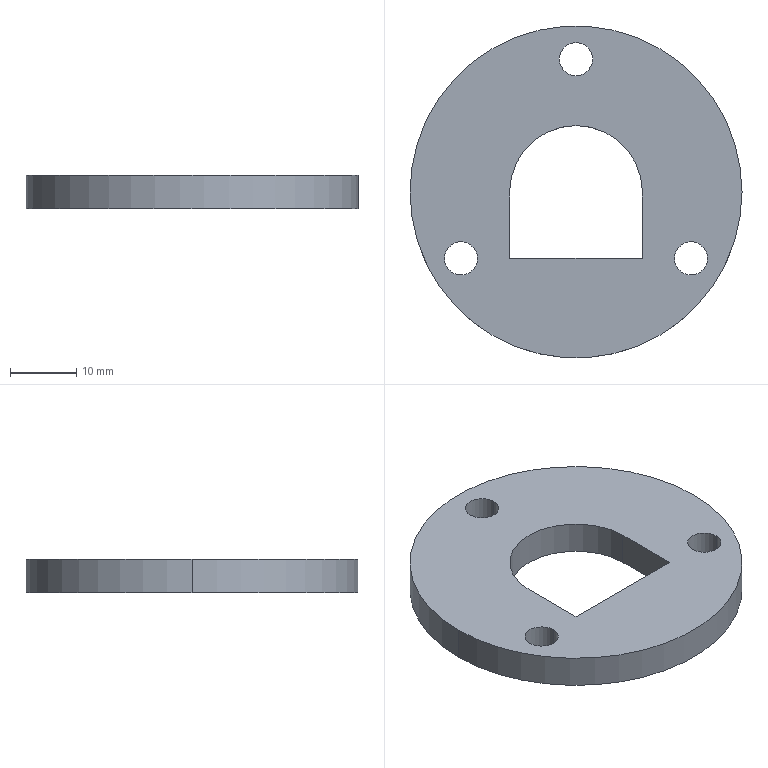Part | SolidWorks | features BaseBody 1 | 1 solid | 14 faces | box 50 x 50 x 5 mm | volume 7738 mm3 | cylinder 9 | plane 5 | commonest cylinder face diameters 5 x6 50 x2 20 x1
STEP:
#1=CARTESIAN_POINT('',(19.821,-10.,0.));
#2=VERTEX_POINT('',#1);
#3=CARTESIAN_POINT('',(14.821,-10.,0.));
#4=VERTEX_POINT('',#3);
#5=CARTESIAN_POINT('',(17.321,-10.,0.));
#6=DIRECTION('',(0.,0.,1.));
#7=DIRECTION('',(-1.,0.,0.));
#8=AXIS2_PLACEMENT_3D('',#5,#6,#7);
#9=CIRCLE('',#8,2.5);
#10=EDGE_CURVE('',#2,#4,#9,.T.);
#11=ORIENTED_EDGE('',*,*,#10,.F.);
#12=CARTESIAN_POINT('',(19.821,-10.,5.));
#13=VERTEX_POINT('',#12);
#14=CARTESIAN_POINT('',(19.821,-10.,5.));
#15=DIRECTION('',(0.,0.,1.));
#16=VECTOR('',#15,1000.);
#17=LINE('',#14,#16);
#18=EDGE_CURVE('',#2,#13,#17,.T.);
#19=ORIENTED_EDGE('',*,*,#18,.T.);
#20=CARTESIAN_POINT('',(14.821,-10.,5.));
#21=VERTEX_POINT('',#20);
#22=CARTESIAN_POINT('',(17.321,-10.,5.));
#23=DIRECTION('',(0.,0.,-1.));
#24=DIRECTION('',(-1.,0.,0.));
#25=AXIS2_PLACEMENT_3D('',#22,#23,#24);
#26=CIRCLE('',#25,2.5);
#27=EDGE_CURVE('',#21,#13,#26,.T.);
#28=ORIENTED_EDGE('',*,*,#27,.F.);
#29=CARTESIAN_POINT('',(14.821,-10.,5.));
#30=DIRECTION('',(0.,0.,1.));
#31=VECTOR('',#30,1000.);
#32=LINE('',#29,#31);
#33=EDGE_CURVE('',#4,#21,#32,.T.);
#34=ORIENTED_EDGE('',*,*,#33,.F.);
#35=EDGE_LOOP('',(#11,#19,#28,#34));
#36=FACE_OUTER_BOUND('',#35,.T.);
#37=CARTESIAN_POINT('',(17.321,-10.,5.));
#38=DIRECTION('',(0.,0.,1.));
#39=DIRECTION('',(-1.,0.,0.));
#40=AXIS2_PLACEMENT_3D('',#37,#38,#39);
#41=CYLINDRICAL_SURFACE('',#40,2.5);
#42=ADVANCED_FACE('',(#36),#41,.F.);
#43=CARTESIAN_POINT('',(-14.821,-10.,0.));
#44=VERTEX_POINT('',#43);
#45=CARTESIAN_POINT('',(-19.821,-10.,0.));
#46=VERTEX_POINT('',#45);
#47=CARTESIAN_POINT('',(-17.321,-10.,0.));
#48=DIRECTION('',(0.,0.,1.));
#49=DIRECTION('',(-1.,0.,0.));
#50=AXIS2_PLACEMENT_3D('',#47,#48,#49);
#51=CIRCLE('',#50,2.5);
#52=EDGE_CURVE('',#44,#46,#51,.T.);
#53=ORIENTED_EDGE('',*,*,#52,.F.);
#54=CARTESIAN_POINT('',(-14.821,-10.,5.));
#55=VERTEX_POINT('',#54);
#56=CARTESIAN_POINT('',(-14.821,-10.,5.));
#57=DIRECTION('',(0.,0.,1.));
#58=VECTOR('',#57,1000.);
#59=LINE('',#56,#58);
#60=EDGE_CURVE('',#44,#55,#59,.T.);
#61=ORIENTED_EDGE('',*,*,#60,.T.);
#62=CARTESIAN_POINT('',(-19.821,-10.,5.));
#63=VERTEX_POINT('',#62);
#64=CARTESIAN_POINT('',(-17.321,-10.,5.));
#65=DIRECTION('',(0.,0.,-1.));
#66=DIRECTION('',(-1.,0.,0.));
#67=AXIS2_PLACEMENT_3D('',#64,#65,#66);
#68=CIRCLE('',#67,2.5);
#69=EDGE_CURVE('',#63,#55,#68,.T.);
#70=ORIENTED_EDGE('',*,*,#69,.F.);
#71=CARTESIAN_POINT('',(-19.821,-10.,5.));
#72=DIRECTION('',(0.,0.,1.));
#73=VECTOR('',#72,1000.);
#74=LINE('',#71,#73);
#75=EDGE_CURVE('',#46,#63,#74,.T.);
#76=ORIENTED_EDGE('',*,*,#75,.F.);
#77=EDGE_LOOP('',(#53,#61,#70,#76));
#78=FACE_OUTER_BOUND('',#77,.T.);
#79=CARTESIAN_POINT('',(-17.321,-10.,5.));
#80=DIRECTION('',(0.,0.,1.));
#81=DIRECTION('',(-1.,0.,0.));
#82=AXIS2_PLACEMENT_3D('',#79,#80,#81);
#83=CYLINDRICAL_SURFACE('',#82,2.5);
#84=ADVANCED_FACE('',(#78),#83,.F.);
#85=CARTESIAN_POINT('',(2.5,20.,0.));
#86=VERTEX_POINT('',#85);
#87=CARTESIAN_POINT('',(-2.5,20.,0.));
#88=VERTEX_POINT('',#87);
#89=CARTESIAN_POINT('',(0.,20.,0.));
#90=DIRECTION('',(0.,0.,1.));
#91=DIRECTION('',(-1.,0.,0.));
#92=AXIS2_PLACEMENT_3D('',#89,#90,#91);
#93=CIRCLE('',#92,2.5);
#94=EDGE_CURVE('',#86,#88,#93,.T.);
#95=ORIENTED_EDGE('',*,*,#94,.F.);
#96=CARTESIAN_POINT('',(2.5,20.,5.));
#97=VERTEX_POINT('',#96);
#98=CARTESIAN_POINT('',(2.5,20.,5.));
#99=DIRECTION('',(0.,0.,1.));
#100=VECTOR('',#99,1000.);
#101=LINE('',#98,#100);
#102=EDGE_CURVE('',#86,#97,#101,.T.);
#103=ORIENTED_EDGE('',*,*,#102,.T.);
#104=CARTESIAN_POINT('',(-2.5,20.,5.));
#105=VERTEX_POINT('',#104);
#106=CARTESIAN_POINT('',(0.,20.,5.));
#107=DIRECTION('',(0.,0.,-1.));
#108=DIRECTION('',(-1.,0.,0.));
#109=AXIS2_PLACEMENT_3D('',#106,#107,#108);
#110=CIRCLE('',#109,2.5);
#111=EDGE_CURVE('',#105,#97,#110,.T.);
#112=ORIENTED_EDGE('',*,*,#111,.F.);
#113=CARTESIAN_POINT('',(-2.5,20.,5.));
#114=DIRECTION('',(0.,0.,1.));
#115=VECTOR('',#114,1000.);
#116=LINE('',#113,#115);
#117=EDGE_CURVE('',#88,#105,#116,.T.);
#118=ORIENTED_EDGE('',*,*,#117,.F.);
#119=EDGE_LOOP('',(#95,#103,#112,#118));
#120=FACE_OUTER_BOUND('',#119,.T.);
#121=CARTESIAN_POINT('',(0.,20.,5.));
#122=DIRECTION('',(0.,0.,1.));
#123=DIRECTION('',(-1.,0.,0.));
#124=AXIS2_PLACEMENT_3D('',#121,#122,#123);
#125=CYLINDRICAL_SURFACE('',#124,2.5);
#126=ADVANCED_FACE('',(#120),#125,.F.);
#127=CARTESIAN_POINT('',(25.,0.,5.));
#128=VERTEX_POINT('',#127);
#129=CARTESIAN_POINT('',(-25.,0.,5.));
#130=VERTEX_POINT('',#129);
#131=CARTESIAN_POINT('',(0.,0.,5.));
#132=DIRECTION('',(0.,0.,1.));
#133=DIRECTION('',(-1.,0.,0.));
#134=AXIS2_PLACEMENT_3D('',#131,#132,#133);
#135=CIRCLE('',#134,25.);
#136=EDGE_CURVE('',#128,#130,#135,.T.);
#137=ORIENTED_EDGE('',*,*,#136,.F.);
#138=CARTESIAN_POINT('',(25.,0.,0.));
#139=VERTEX_POINT('',#138);
#140=CARTESIAN_POINT('',(25.,0.,0.));
#141=DIRECTION('',(0.,0.,-1.));
#142=VECTOR('',#141,1000.);
#143=LINE('',#140,#142);
#144=EDGE_CURVE('',#128,#139,#143,.T.);
#145=ORIENTED_EDGE('',*,*,#144,.T.);
#146=CARTESIAN_POINT('',(-25.,0.,0.));
#147=VERTEX_POINT('',#146);
#148=CARTESIAN_POINT('',(0.,0.,0.));
#149=DIRECTION('',(0.,0.,-1.));
#150=DIRECTION('',(-1.,0.,0.));
#151=AXIS2_PLACEMENT_3D('',#148,#149,#150);
#152=CIRCLE('',#151,25.);
#153=EDGE_CURVE('',#147,#139,#152,.T.);
#154=ORIENTED_EDGE('',*,*,#153,.F.);
#155=CARTESIAN_POINT('',(-25.,0.,0.));
#156=DIRECTION('',(0.,0.,-1.));
#157=VECTOR('',#156,1000.);
#158=LINE('',#155,#157);
#159=EDGE_CURVE('',#130,#147,#158,.T.);
#160=ORIENTED_EDGE('',*,*,#159,.F.);
#161=EDGE_LOOP('',(#137,#145,#154,#160));
#162=FACE_OUTER_BOUND('',#161,.T.);
#163=CARTESIAN_POINT('',(0.,0.,0.));
#164=DIRECTION('',(0.,0.,-1.));
#165=DIRECTION('',(-1.,0.,0.));
#166=AXIS2_PLACEMENT_3D('',#163,#164,#165);
#167=CYLINDRICAL_SURFACE('',#166,25.);
#168=ADVANCED_FACE('',(#162),#167,.T.);
#169=CARTESIAN_POINT('',(10.,0.,0.));
#170=VERTEX_POINT('',#169);
#171=CARTESIAN_POINT('',(-10.,0.,0.));
#172=VERTEX_POINT('',#171);
#173=CARTESIAN_POINT('',(0.,0.,0.));
#174=DIRECTION('',(0.,0.,1.));
#175=DIRECTION('',(1.,0.,0.));
#176=AXIS2_PLACEMENT_3D('',#173,#174,#175);
#177=CIRCLE('',#176,10.);
#178=EDGE_CURVE('',#170,#172,#177,.T.);
#179=ORIENTED_EDGE('',*,*,#178,.F.);
#180=CARTESIAN_POINT('',(10.,0.,5.));
#181=VERTEX_POINT('',#180);
#182=CARTESIAN_POINT('',(10.,0.,5.));
#183=DIRECTION('',(0.,0.,-1.));
#184=VECTOR('',#183,1000.);
#185=LINE('',#182,#184);
#186=EDGE_CURVE('',#181,#170,#185,.T.);
#187=ORIENTED_EDGE('',*,*,#186,.F.);
#188=CARTESIAN_POINT('',(-10.,0.,5.));
#189=VERTEX_POINT('',#188);
#190=CARTESIAN_POINT('',(0.,0.,5.));
#191=DIRECTION('',(0.,0.,-1.));
#192=DIRECTION('',(1.,0.,0.));
#193=AXIS2_PLACEMENT_3D('',#190,#191,#192);
#194=CIRCLE('',#193,10.);
#195=EDGE_CURVE('',#189,#181,#194,.T.);
#196=ORIENTED_EDGE('',*,*,#195,.F.);
#197=CARTESIAN_POINT('',(-10.,0.,5.));
#198=DIRECTION('',(0.,0.,-1.));
#199=VECTOR('',#198,1000.);
#200=LINE('',#197,#199);
#201=EDGE_CURVE('',#189,#172,#200,.T.);
#202=ORIENTED_EDGE('',*,*,#201,.T.);
#203=EDGE_LOOP('',(#179,#187,#196,#202));
#204=FACE_OUTER_BOUND('',#203,.T.);
#205=CARTESIAN_POINT('',(0.,0.,5.));
#206=DIRECTION('',(0.,0.,1.));
#207=DIRECTION('',(1.,0.,0.));
#208=AXIS2_PLACEMENT_3D('',#205,#206,#207);
#209=CYLINDRICAL_SURFACE('',#208,10.);
#210=ADVANCED_FACE('',(#204),#209,.F.);
#211=CARTESIAN_POINT('',(-10.,-10.,0.));
#212=VERTEX_POINT('',#211);
#213=CARTESIAN_POINT('',(-10.,-5.,0.));
#214=DIRECTION('',(0.,-1.,0.));
#215=VECTOR('',#214,1000.);
#216=LINE('',#213,#215);
#217=EDGE_CURVE('',#172,#212,#216,.T.);
#218=ORIENTED_EDGE('',*,*,#217,.F.);
#219=ORIENTED_EDGE('',*,*,#201,.F.);
#220=CARTESIAN_POINT('',(-10.,-10.,5.));
#221=VERTEX_POINT('',#220);
#222=CARTESIAN_POINT('',(-10.,-5.,5.));
#223=DIRECTION('',(0.,1.,0.));
#224=VECTOR('',#223,1000.);
#225=LINE('',#222,#224);
#226=EDGE_CURVE('',#221,#189,#225,.T.);
#227=ORIENTED_EDGE('',*,*,#226,.F.);
#228=CARTESIAN_POINT('',(-10.,-10.,5.));
#229=DIRECTION('',(0.,0.,-1.));
#230=VECTOR('',#229,1000.);
#231=LINE('',#228,#230);
#232=EDGE_CURVE('',#221,#212,#231,.T.);
#233=ORIENTED_EDGE('',*,*,#232,.T.);
#234=EDGE_LOOP('',(#218,#219,#227,#233));
#235=FACE_OUTER_BOUND('',#234,.T.);
#236=CARTESIAN_POINT('',(-10.,-10.,5.));
#237=DIRECTION('',(-1.,0.,0.));
#238=DIRECTION('',(0.,0.,1.));
#239=AXIS2_PLACEMENT_3D('',#236,#237,#238);
#240=PLANE('',#239);
#241=ADVANCED_FACE('',(#235),#240,.F.);
#242=CARTESIAN_POINT('',(10.,-10.,0.));
#243=VERTEX_POINT('',#242);
#244=CARTESIAN_POINT('',(5.,-10.,0.));
#245=DIRECTION('',(1.,0.,0.));
#246=VECTOR('',#245,1000.);
#247=LINE('',#244,#246);
#248=EDGE_CURVE('',#212,#243,#247,.T.);
#249=ORIENTED_EDGE('',*,*,#248,.F.);
#250=ORIENTED_EDGE('',*,*,#232,.F.);
#251=CARTESIAN_POINT('',(10.,-10.,5.));
#252=VERTEX_POINT('',#251);
#253=CARTESIAN_POINT('',(5.,-10.,5.));
#254=DIRECTION('',(-1.,0.,0.));
#255=VECTOR('',#254,1000.);
#256=LINE('',#253,#255);
#257=EDGE_CURVE('',#252,#221,#256,.T.);
#258=ORIENTED_EDGE('',*,*,#257,.F.);
#259=CARTESIAN_POINT('',(10.,-10.,5.));
#260=DIRECTION('',(0.,0.,-1.));
#261=VECTOR('',#260,1000.);
#262=LINE('',#259,#261);
#263=EDGE_CURVE('',#252,#243,#262,.T.);
#264=ORIENTED_EDGE('',*,*,#263,.T.);
#265=EDGE_LOOP('',(#249,#250,#258,#264));
#266=FACE_OUTER_BOUND('',#265,.T.);
#267=CARTESIAN_POINT('',(10.,-10.,5.));
#268=DIRECTION('',(0.,-1.,0.));
#269=DIRECTION('',(0.,0.,-1.));
#270=AXIS2_PLACEMENT_3D('',#267,#268,#269);
#271=PLANE('',#270);
#272=ADVANCED_FACE('',(#266),#271,.F.);
#273=CARTESIAN_POINT('',(10.,0.,0.));
#274=DIRECTION('',(0.,1.,0.));
#275=VECTOR('',#274,1000.);
#276=LINE('',#273,#275);
#277=EDGE_CURVE('',#243,#170,#276,.T.);
#278=ORIENTED_EDGE('',*,*,#277,.F.);
#279=ORIENTED_EDGE('',*,*,#263,.F.);
#280=CARTESIAN_POINT('',(10.,0.,5.));
#281=DIRECTION('',(0.,-1.,0.));
#282=VECTOR('',#281,1000.);
#283=LINE('',#280,#282);
#284=EDGE_CURVE('',#181,#252,#283,.T.);
#285=ORIENTED_EDGE('',*,*,#284,.F.);
#286=ORIENTED_EDGE('',*,*,#186,.T.);
#287=EDGE_LOOP('',(#278,#279,#285,#286));
#288=FACE_OUTER_BOUND('',#287,.T.);
#289=CARTESIAN_POINT('',(10.,0.,5.));
#290=DIRECTION('',(1.,0.,0.));
#291=DIRECTION('',(0.,1.,0.));
#292=AXIS2_PLACEMENT_3D('',#289,#290,#291);
#293=PLANE('',#292);
#294=ADVANCED_FACE('',(#288),#293,.F.);
#295=CARTESIAN_POINT('',(17.321,-10.,0.));
#296=DIRECTION('',(0.,0.,1.));
#297=DIRECTION('',(-1.,0.,0.));
#298=AXIS2_PLACEMENT_3D('',#295,#296,#297);
#299=CIRCLE('',#298,2.5);
#300=EDGE_CURVE('',#4,#2,#299,.T.);
#301=ORIENTED_EDGE('',*,*,#300,.T.);
#302=ORIENTED_EDGE('',*,*,#10,.T.);
#303=EDGE_LOOP('',(#301,#302));
#304=FACE_BOUND('',#303,.T.);
#305=CARTESIAN_POINT('',(-17.321,-10.,0.));
#306=DIRECTION('',(0.,0.,1.));
#307=DIRECTION('',(-1.,0.,0.));
#308=AXIS2_PLACEMENT_3D('',#305,#306,#307);
#309=CIRCLE('',#308,2.5);
#310=EDGE_CURVE('',#46,#44,#309,.T.);
#311=ORIENTED_EDGE('',*,*,#310,.T.);
#312=ORIENTED_EDGE('',*,*,#52,.T.);
#313=EDGE_LOOP('',(#311,#312));
#314=FACE_BOUND('',#313,.T.);
#315=CARTESIAN_POINT('',(0.,20.,0.));
#316=DIRECTION('',(0.,0.,1.));
#317=DIRECTION('',(-1.,0.,0.));
#318=AXIS2_PLACEMENT_3D('',#315,#316,#317);
#319=CIRCLE('',#318,2.5);
#320=EDGE_CURVE('',#88,#86,#319,.T.);
#321=ORIENTED_EDGE('',*,*,#320,.T.);
#322=ORIENTED_EDGE('',*,*,#94,.T.);
#323=EDGE_LOOP('',(#321,#322));
#324=FACE_BOUND('',#323,.T.);
#325=ORIENTED_EDGE('',*,*,#248,.T.);
#326=ORIENTED_EDGE('',*,*,#277,.T.);
#327=ORIENTED_EDGE('',*,*,#178,.T.);
#328=ORIENTED_EDGE('',*,*,#217,.T.);
#329=EDGE_LOOP('',(#325,#326,#327,#328));
#330=FACE_BOUND('',#329,.T.);
#331=ORIENTED_EDGE('',*,*,#153,.T.);
#332=CARTESIAN_POINT('',(0.,0.,0.));
#333=DIRECTION('',(0.,0.,-1.));
#334=DIRECTION('',(-1.,0.,0.));
#335=AXIS2_PLACEMENT_3D('',#332,#333,#334);
#336=CIRCLE('',#335,25.);
#337=EDGE_CURVE('',#139,#147,#336,.T.);
#338=ORIENTED_EDGE('',*,*,#337,.T.);
#339=EDGE_LOOP('',(#331,#338));
#340=FACE_OUTER_BOUND('',#339,.T.);
#341=CARTESIAN_POINT('',(0.,0.,0.));
#342=DIRECTION('',(0.,0.,1.));
#343=DIRECTION('',(1.,0.,0.));
#344=AXIS2_PLACEMENT_3D('',#341,#342,#343);
#345=PLANE('',#344);
#346=ADVANCED_FACE('',(#304,#314,#324,#330,#340),#345,.F.);
#347=ORIENTED_EDGE('',*,*,#27,.T.);
#348=CARTESIAN_POINT('',(17.321,-10.,5.));
#349=DIRECTION('',(0.,0.,-1.));
#350=DIRECTION('',(-1.,0.,0.));
#351=AXIS2_PLACEMENT_3D('',#348,#349,#350);
#352=CIRCLE('',#351,2.5);
#353=EDGE_CURVE('',#13,#21,#352,.T.);
#354=ORIENTED_EDGE('',*,*,#353,.T.);
#355=EDGE_LOOP('',(#347,#354));
#356=FACE_BOUND('',#355,.T.);
#357=ORIENTED_EDGE('',*,*,#69,.T.);
#358=CARTESIAN_POINT('',(-17.321,-10.,5.));
#359=DIRECTION('',(0.,0.,-1.));
#360=DIRECTION('',(-1.,0.,0.));
#361=AXIS2_PLACEMENT_3D('',#358,#359,#360);
#362=CIRCLE('',#361,2.5);
#363=EDGE_CURVE('',#55,#63,#362,.T.);
#364=ORIENTED_EDGE('',*,*,#363,.T.);
#365=EDGE_LOOP('',(#357,#364));
#366=FACE_BOUND('',#365,.T.);
#367=ORIENTED_EDGE('',*,*,#111,.T.);
#368=CARTESIAN_POINT('',(0.,20.,5.));
#369=DIRECTION('',(0.,0.,-1.));
#370=DIRECTION('',(-1.,0.,0.));
#371=AXIS2_PLACEMENT_3D('',#368,#369,#370);
#372=CIRCLE('',#371,2.5);
#373=EDGE_CURVE('',#97,#105,#372,.T.);
#374=ORIENTED_EDGE('',*,*,#373,.T.);
#375=EDGE_LOOP('',(#367,#374));
#376=FACE_BOUND('',#375,.T.);
#377=ORIENTED_EDGE('',*,*,#257,.T.);
#378=ORIENTED_EDGE('',*,*,#226,.T.);
#379=ORIENTED_EDGE('',*,*,#195,.T.);
#380=ORIENTED_EDGE('',*,*,#284,.T.);
#381=EDGE_LOOP('',(#377,#378,#379,#380));
#382=FACE_BOUND('',#381,.T.);
#383=CARTESIAN_POINT('',(0.,0.,5.));
#384=DIRECTION('',(0.,0.,1.));
#385=DIRECTION('',(-1.,0.,0.));
#386=AXIS2_PLACEMENT_3D('',#383,#384,#385);
#387=CIRCLE('',#386,25.);
#388=EDGE_CURVE('',#130,#128,#387,.T.);
#389=ORIENTED_EDGE('',*,*,#388,.T.);
#390=ORIENTED_EDGE('',*,*,#136,.T.);
#391=EDGE_LOOP('',(#389,#390));
#392=FACE_OUTER_BOUND('',#391,.T.);
#393=CARTESIAN_POINT('',(0.,0.,5.));
#394=DIRECTION('',(0.,0.,1.));
#395=DIRECTION('',(1.,0.,0.));
#396=AXIS2_PLACEMENT_3D('',#393,#394,#395);
#397=PLANE('',#396);
#398=ADVANCED_FACE('',(#356,#366,#376,#382,#392),#397,.T.);
#399=ORIENTED_EDGE('',*,*,#144,.F.);
#400=ORIENTED_EDGE('',*,*,#388,.F.);
#401=ORIENTED_EDGE('',*,*,#159,.T.);
#402=ORIENTED_EDGE('',*,*,#337,.F.);
#403=EDGE_LOOP('',(#399,#400,#401,#402));
#404=FACE_OUTER_BOUND('',#403,.T.);
#405=CARTESIAN_POINT('',(0.,0.,0.));
#406=DIRECTION('',(0.,0.,-1.));
#407=DIRECTION('',(-1.,0.,0.));
#408=AXIS2_PLACEMENT_3D('',#405,#406,#407);
#409=CYLINDRICAL_SURFACE('',#408,25.);
#410=ADVANCED_FACE('',(#404),#409,.T.);
#411=ORIENTED_EDGE('',*,*,#102,.F.);
#412=ORIENTED_EDGE('',*,*,#320,.F.);
#413=ORIENTED_EDGE('',*,*,#117,.T.);
#414=ORIENTED_EDGE('',*,*,#373,.F.);
#415=EDGE_LOOP('',(#411,#412,#413,#414));
#416=FACE_OUTER_BOUND('',#415,.T.);
#417=CARTESIAN_POINT('',(0.,20.,5.));
#418=DIRECTION('',(0.,0.,1.));
#419=DIRECTION('',(-1.,0.,0.));
#420=AXIS2_PLACEMENT_3D('',#417,#418,#419);
#421=CYLINDRICAL_SURFACE('',#420,2.5);
#422=ADVANCED_FACE('',(#416),#421,.F.);
#423=ORIENTED_EDGE('',*,*,#60,.F.);
#424=ORIENTED_EDGE('',*,*,#310,.F.);
#425=ORIENTED_EDGE('',*,*,#75,.T.);
#426=ORIENTED_EDGE('',*,*,#363,.F.);
#427=EDGE_LOOP('',(#423,#424,#425,#426));
#428=FACE_OUTER_BOUND('',#427,.T.);
#429=CARTESIAN_POINT('',(-17.321,-10.,5.));
#430=DIRECTION('',(0.,0.,1.));
#431=DIRECTION('',(-1.,0.,0.));
#432=AXIS2_PLACEMENT_3D('',#429,#430,#431);
#433=CYLINDRICAL_SURFACE('',#432,2.5);
#434=ADVANCED_FACE('',(#428),#433,.F.);
#435=ORIENTED_EDGE('',*,*,#18,.F.);
#436=ORIENTED_EDGE('',*,*,#300,.F.);
#437=ORIENTED_EDGE('',*,*,#33,.T.);
#438=ORIENTED_EDGE('',*,*,#353,.F.);
#439=EDGE_LOOP('',(#435,#436,#437,#438));
#440=FACE_OUTER_BOUND('',#439,.T.);
#441=CARTESIAN_POINT('',(17.321,-10.,5.));
#442=DIRECTION('',(0.,0.,1.));
#443=DIRECTION('',(-1.,0.,0.));
#444=AXIS2_PLACEMENT_3D('',#441,#442,#443);
#445=CYLINDRICAL_SURFACE('',#444,2.5);
#446=ADVANCED_FACE('',(#440),#445,.F.);
#447=CLOSED_SHELL('',(#42,#84,#126,#168,#210,#241,#272,#294,#346,#398,#410,#422,#434,#446));
#448=MANIFOLD_SOLID_BREP('',#447);
#449=CARTESIAN_POINT('',(0.,0.,0.));
#450=DIRECTION('',(0.,0.,1.));
#451=DIRECTION('',(1.,0.,0.));
#452=AXIS2_PLACEMENT_3D('',#449,#450,#451);
#453=(LENGTH_UNIT()NAMED_UNIT(*)SI_UNIT(.MILLI.,.METRE.));
#454=UNCERTAINTY_MEASURE_WITH_UNIT(LENGTH_MEASURE(0.00001),#453,'','');
#455=(NAMED_UNIT(*)PLANE_ANGLE_UNIT()SI_UNIT($,.RADIAN.));
#456=(NAMED_UNIT(*)SI_UNIT($,.STERADIAN.)SOLID_ANGLE_UNIT());
#457=(GEOMETRIC_REPRESENTATION_CONTEXT(3)GLOBAL_UNCERTAINTY_ASSIGNED_CONTEXT((#454))GLOBAL_UNIT_ASSIGNED_CONTEXT((#453,#455,#456))REPRESENTATION_CONTEXT('',''));
#458=ADVANCED_BREP_SHAPE_REPRESENTATION('',(#448,#452),#457);